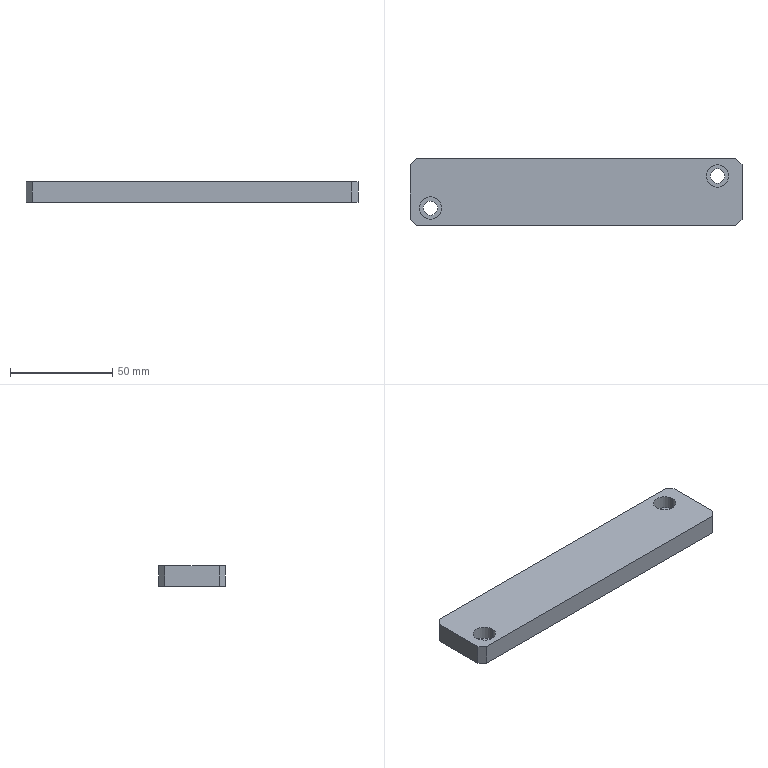Part | STEP file | 1_id538_x_t | 1 solid | 29 faces | box 162.45 x 32.752 x 10 mm | volume 49655 mm3 | plane 15 | cylinder 14 | commonest cylinder face diameters 12 x6 7 x4 11 x4